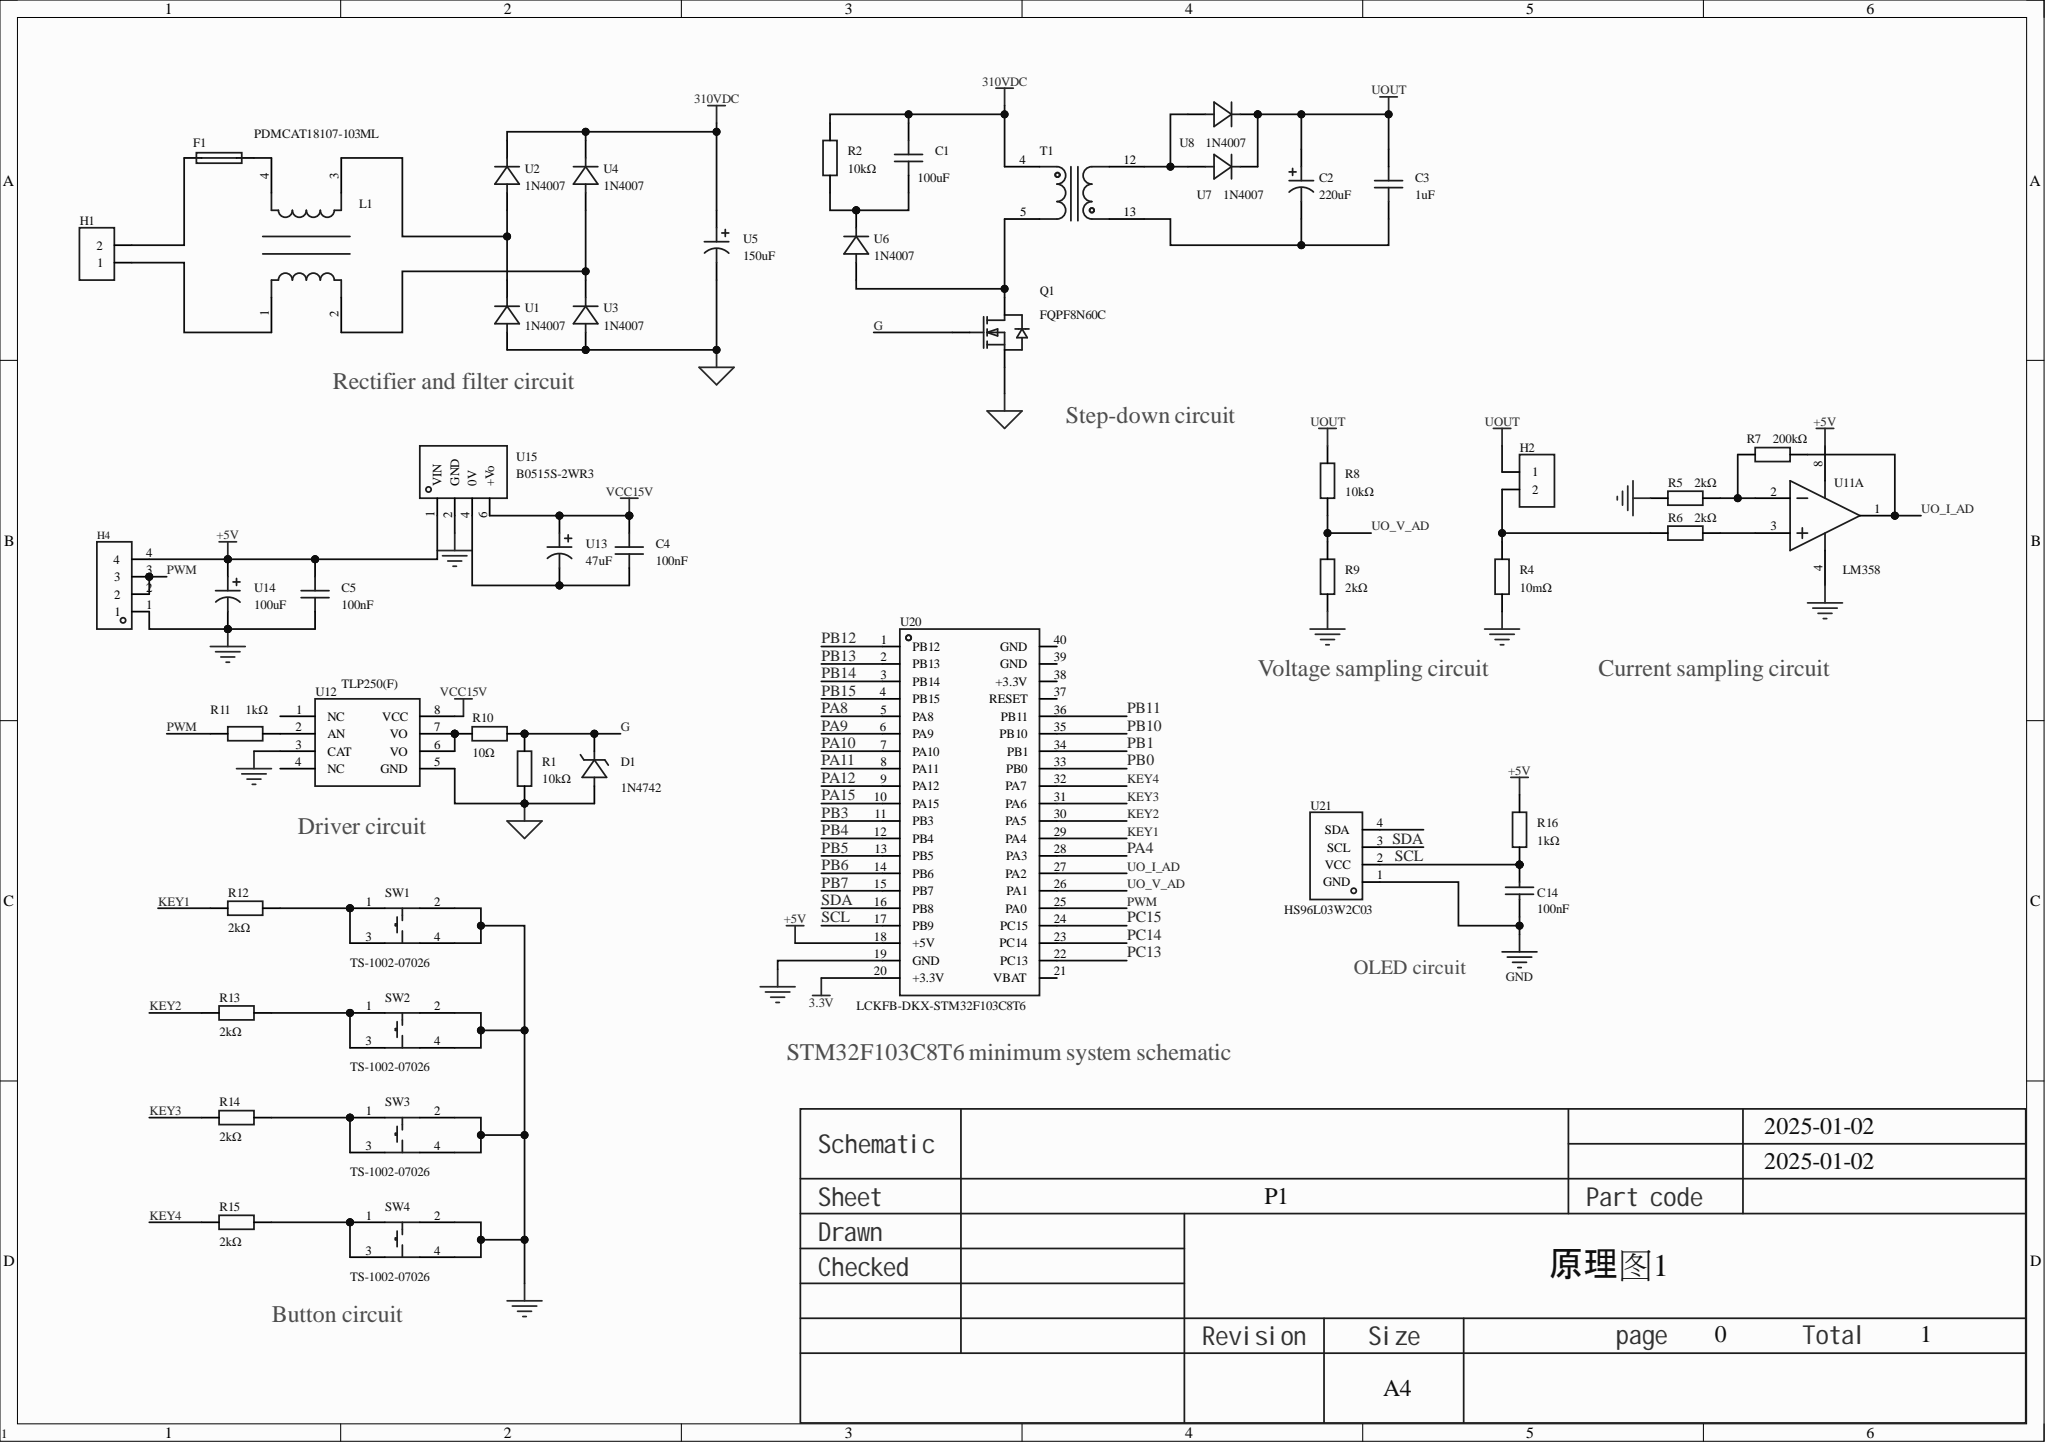Circuit board | Altium Designer | 48 parts | 36 nets
Bill of materials:
Comment,Description,Designator,Footprint,LibRef,Quantity
"100uF","Capacitance:100nF;Tolerance:±5%;Rated voltage:630V;Operating temperature:-40℃~+100℃;","C1","CAP-TH_L12.0-W5.5-P10.00-D1.0","KP104J2J1006","1"
"220uF","Capacitance:220uF;Tolerance:±20%;Rated voltage:50V;Ripple current:350mA@120kHz;ESR:-;","C2","CAP-TH_BD8.0-P3.50-D0.6-FD","01EC3470","1"
"1uF","Capacitance:1uF;Tolerance:±10%;Rated voltage:50V;Temperature coefficient:X7R;","C3","CAP-TH_L5.8-W3.6-P5.0-D0.6","178MU0005","1"
"100nF","Capacitance:100nF;Tolerance:±20%;Rated voltage:50V;Temperature coefficient:Y5V;","C4, C5","CAP-TH_L5.0-W2.5-P5.00-D1.0","CC1H104MC1FD3F6C10MF","2"
"100nF","","C14","C0805","CC0805KRX7R9BB104","1"
"1N4742","Diode configuration:Single;Zener voltage (nominal):12V;Zener voltage (range):11.45V~12.95V;Power:1W;Tolerance:±5%;","D1","DO-41_BD2.4-L4.7-P8.70-D0.8-FD","1N4742","1"
"5F0.2R1","Type:glass tube fuse;Rated current:2A;","F1","FUSE-SMD_5-20MM","5F0.2R1","1"
"","","H1, H2","HDR-TH_2P-P2.54-V-F","HDR-F_2.54_1x2P","2"
"","","H4","HDR-TH_4P-P2.54-V-F","HDR-F_2.54_1x4P","1"
"PDMCAT18107-103ML","Lines:2;Inductance @ frequency:10mH@1kHz;DC resistance (DCR):55mΩ;","L1","IND-TH_4P-L22.0-W12.0-TR","PDMCAT18107-103ML","1"
"FQPF8N60C","Type:1 N-channel;Drain-source voltage (Vdss):600V;Continuous drain current (Id):7.5A;On-resistance (RDS(on)@Vgs,Id):1.2Ω@10V,3.75A;Power (Pd):48W;Gate threshold voltage (Vgs(th)@Id):4V@250uA;","Q1","TO-220F-3_L10.2-W4.9-P2.54-L","FQPF8N60C","1"
"10kΩ","","R1, R8","Res_1/4W","Res_AXIAL-1/4W","2"
"10kΩ","","R2","Res_1W","Res_AXIAL-1W","1"
"10mΩ","","R4","Res_1/4W","Res_AXIAL-1/4W","1"
"2kΩ","","R5, R6, R9, R12, R13, R14, R15","Res_1/4W","Res_AXIAL-1/4W","7"
"200kΩ","","R7","Res_1/4W","Res_AXIAL-1/4W","1"
"10Ω","","R10","Res_1/4W","Res_AXIAL-1/4W","1"
"1kΩ","","R11, R16","Res_1/4W","Res_AXIAL-1/4W","2"
"TS-1002-07026","Circuit structure:Single-pole single-throw;Button shape:Round button;Mounting style:Through-hole;Switch length:6mm;Switch width:6mm;Switch height:7mm;Contact current:50mA;Rated voltage (DC):12V;With LED:-;Mechanical life:-;","SW1, SW2, SW3, SW4","SW-TH_4P-L6.0-W6.0-P4.50-LS6.5","TS-1002-07026","4"
"","Primary voltage:-;Secondary voltage:-;Output current:-;Power:2W;","T1","dip2_8_5mm_35MM","T220Vto18V","1"
"1N4007","","U1, U2, U3, U4, U6, U7, U8","DO-41_BD2.4-L4.7-P8.70-D0.6-RD","1N4007_C5261026","7"
"150uF","Capacitance:150uF;Rated voltage:400V;","U5","CAP-TH_BD18.0-P7.50-D0.8-FD","CD1101572GM1836VFL","1"
"LM358","","U11","DIP-8_L9.8-W6.4-P2.54-LS7.6-BL","LM358_C5157924","1"
"TLP250(F)","Input type:DC;Supply voltage:10V~35V;Common-mode transient immunity CMTI:5kV/us;Propagation delay tpLH/tpHL:500ns;500ns;","U12","DIP-8_L9.4-W6.4-P2.54-LS9.1-BL","TLP250(F)","1"
"47uF","Capacitance:47uF;Tolerance:±20%;Rated voltage:25V;Ripple current:80mA@120kHz;ESR:-;","U13","CAP-TH_BD5.0-P2.00-D0.5-FD","KM1E470M0507","1"
"100uF","Capacitance:47uF;Tolerance:±20%;Rated voltage:25V;Ripple current:80mA@120kHz;ESR:-;","U14","CAP-TH_BD5.0-P2.00-D0.5-FD","KM1E470M0507","1"
"B0515S-2WR3","100% domestically produced. B1215S-2WR3 is designed for board-level power systems that need an isolated voltage separate from the input supply. Suitable for: 1) input supply with stable voltage (voltage variation ±10%Vin); 2) input-output isolation required (isolation voltage =1500VDC); 3) low output voltage stability requirement; 4) typical applications: pure digital circuits, general low-frequency analog circuits, relay drive circuits, data exchange circuits. Features: fixed voltage input, isolated unregulated output, 2W, isolation voltage: 1500VDC, efficiency: up to 84%,","U15","SIP-4_L19.5-W7.0-P2.54-L","B1215S-2WR3_C5369480","1"
"LCKFB-DKX-STM32F103C8T6","","U20","CONN-TH_L53.3-W22.9_STM32F103C8T6-CARD","LCKFB-DKX-STM32F103C8T6","1"
"HS96L03W2C03","Main controller chip:SSD1315;Interface type:I2C;Size (inch):0.96;Pixel resolution:128x64;","U21","OLED-TH_L27.8-W27.2-P2.54_C9900033791","HS96L03W2C03","1"
Netlist (Protel format):
[
C1
CAP-TH_L12.0-W5.5-P10.00-D1.0
100uF



]
[
C2
CAP-TH_BD8.0-P3.50-D0.6-FD
220uF



]
[
C3
CAP-TH_L5.8-W3.6-P5.0-D0.6
1uF



]
[
C4
CAP-TH_L5.0-W2.5-P5.00-D1.0
100nF



]
[
C5
CAP-TH_L5.0-W2.5-P5.00-D1.0
100nF



]
[
C14
C0805
100nF



]
[
D1
DO-41_BD2.4-L4.7-P8.70-D0.8-FD
1N4742



]
[
F1
FUSE-SMD_5-20MM
5F.2000210000R1



]
[
H1
HDR-TH_2P-P2.54-V-F




]
[
H2
HDR-TH_2P-P2.54-V-F




]
[
H4
HDR-TH_4P-P2.54-V-F




]
[
L1
IND-TH_4P-L22.0-W12.0-TR
PDMCAT18107-103ML



]
[
Q1
TO-220F-3_L10.2-W4.9-P2.54-L
FQPF8N60C



]
[
R1
Res_1/4W
10kΩ



]
[
R2
Res_1W
10kΩ



]
[
R4
Res_1/4W
10mΩ



]
[
R5
Res_1/4W
2kΩ



]
[
R6
Res_1/4W
2kΩ



]
[
R7
Res_1/4W
200kΩ



]
[
R8
Res_1/4W
10kΩ



]
[
R9
Res_1/4W
2kΩ



]
[
R10
Res_1/4W
10Ω



]
[
R11
Res_1/4W
1kΩ



]
[
R12
Res_1/4W
2kΩ



]
[
R13
Res_1/4W
2kΩ



]
[
R14
Res_1/4W
2kΩ



]
[
R15
Res_1/4W
2kΩ



]
[
R16
Res_1/4W
1kΩ



]
[
SW1
SW-TH_4P-L6.0-W6.0-P4.50-LS6.5
TS-1002-07026



]
[
SW2
SW-TH_4P-L6.0-W6.0-P4.50-LS6.5
TS-1002-07026



]
[
SW3
SW-TH_4P-L6.0-W6.0-P4.50-LS6.5
TS-1002-07026



]
[
SW4
SW-TH_4P-L6.0-W6.0-P4.50-LS6.5
TS-1002-07026



]
[
T1
dip2_8_5mm_35MM




]
[
U1
DO-41_BD2.4-L4.7-P8.70-D0.6-RD
1N4007



]
[
U2
DO-41_BD2.4-L4.7-P8.70-D0.6-RD
1N4007



]
[
U3
DO-41_BD2.4-L4.7-P8.70-D0.6-RD
1N4007



]
[
U4
DO-41_BD2.4-L4.7-P8.70-D0.6-RD
1N4007



]
[
U5
CAP-TH_BD18.0-P7.50-D0.8-FD
150uF



]
[
U6
DO-41_BD2.4-L4.7-P8.70-D0.6-RD
1N4007



]
[
U7
DO-41_BD2.4-L4.7-P8.70-D0.6-RD
1N4007



]
[
U8
DO-41_BD2.4-L4.7-P8.70-D0.6-RD
1N4007



]
[
U11
DIP-8_L9.8-W6.4-P2.54-LS7.6-BL
LM358



]
[
U12
DIP-8_L9.4-W6.4-P2.54-LS9.1-BL
TLP250(F)



]
[
U13
CAP-TH_BD5.0-P2.00-D0.5-FD
47uF



]
[
U14
CAP-TH_BD5.0-P2.00-D0.5-FD
100uF



]
[
U15
SIP-4_L19.5-W7.0-P2.54-L
B0515S-2WR3



]
[
U20
CONN-TH_L53.3-W22.9_STM32F103C8T6-CARD
LCKFB-DKX-STM32F103C8T6



]
[
U21
OLED-TH_L27.8-W27.2-P2.54_C9900033791
HS96L03W2C03



]
(
VCC15V
C4-1
U12-8
U13-1
U15-6
)
(
UOUT
C2-1
C3-2
H2-1
R8-2
U7-1
U8-1
)
(
UO_V_AD
R8-1
R9-2
U20-26
)
(
UO_I_AD
R7-2
U11-1
U20-27
)
(
SDA
U20-16
U21-4
)
(
SCL
U20-17
U21-3
)
(
PWM
H4-2
H4-3
R11-1
U20-25
)
(
NetT1_12
T1-12
U7-2
U8-2
)
(
NetR15_1
R15-1
SW4-1
SW4-3
)
(
NetR14_1
R14-1
SW3-1
SW3-3
)
(
NetR13_1
R13-1
SW2-1
SW2-3
)
(
NetR12_1
R12-1
SW1-1
SW1-3
)
(
NetR11_2
R11-2
U12-2
)
(
NetR10_1
R10-1
U12-6
U12-7
)
(
NetR6_2
R6-2
U11-3
)
(
NetR5_2
R5-2
R7-1
U11-2
)
(
NetQ1_2
Q1-2
T1-5
U6-2
)
(
NetL1_3
L1-3
U1-1
U2-2
)
(
NetL1_2
L1-2
U3-1
U4-2
)
(
NetH2_2
H2-2
R4-2
R6-1
)
(
NetH1_1
H1-1
L1-1
)
(
NetF1_2
F1-2
L1-4
)
(
NetF1_1
F1-1
H1-2
)
(
NetC14_2
C14-2
R16-1
U21-2
)
(
NetC4_2
C4-2
U13-2
U15-4
)
(
NetC2_2
C2-2
C3-1
T1-13
)
(
NetC1_1
C1-1
R2-1
U6-1
)
(
KEY4
R15-2
U20-32
)
(
KEY3
R14-2
U20-31
)
(
KEY2
R13-2
U20-30
)
(
KEY1
R12-2
U20-29
)
(
GND
C5-2
C14-1
H4-1
R4-1
R5-1
R9-1
SW1-2
SW1-4
SW2-2
SW2-4
SW3-2
SW3-4
SW4-2
SW4-4
U11-4
U12-3
U14-2
U15-2
U20-19
U21-1
)
(
G
D1-2
Q1-1
R1-1
R10-2
)
(
AGND
D1-1
Q1-3
R1-2
U1-2
U3-2
U5-2
U12-5
)
(
+5V
C5-1
H4-4
R16-2
U11-8
U14-1
U15-1
U20-18
)
(
310VDC
C1-2
R2-2
T1-4
U2-1
U4-1
U5-1
)